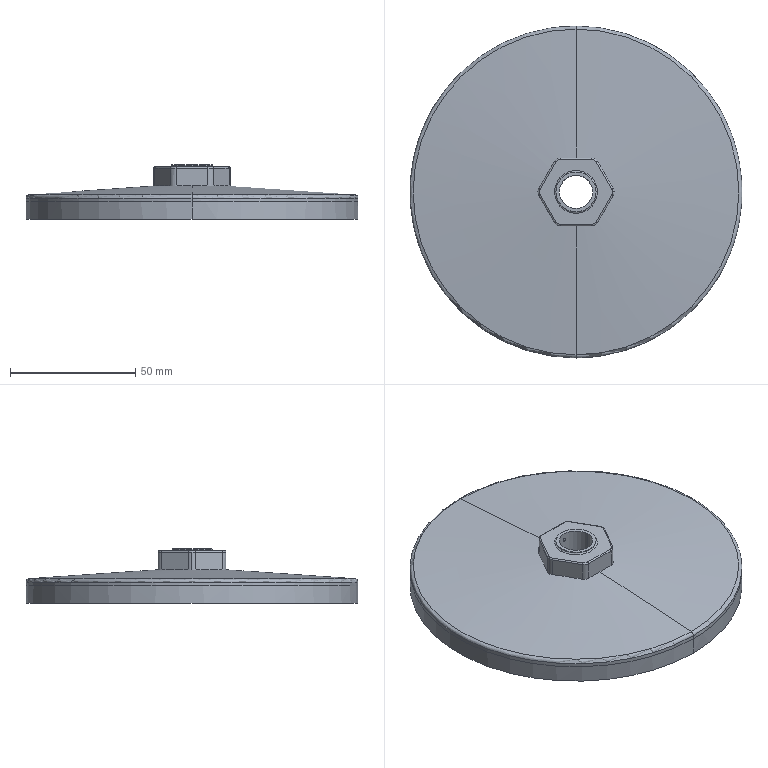Part | SolidWorks | features Fillet 3, ICE 3, BossThin 2, Extrusion 1, Revolution 1, Scale 1 | 1 solid | 48 faces | box 132.316 x 132.316 x 21.819 mm | volume 70046 mm3 | cylinder 25 | torus 11 | plane 10 | cone 2 | commonest cylinder face diameters 5.4 x7 1.08 x6 1.35 x2 13.277 x2 15.977 x2 126.316 x2